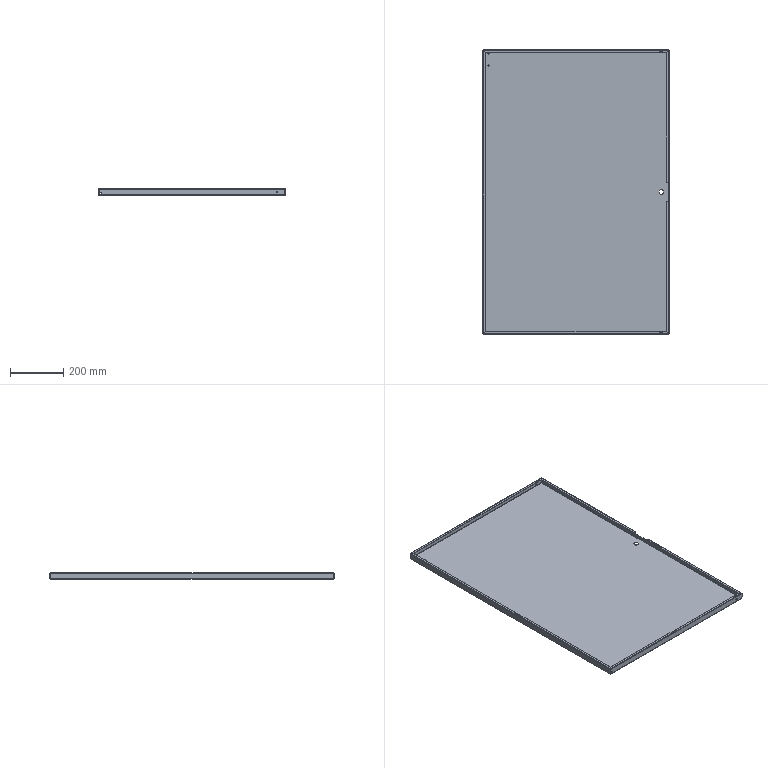Part | SolidWorks | features Cut 4, EdgeFlange 2, ICE 2, Fillet 1, FlatPattern 1, LPattern 1, MirrorPattern 1, SMBaseFlange 1, SheetMetal 1 | 1 solid | 110 faces | box 700 x 1066 x 25 mm | volume 1278991 mm3 | plane 52 | cylinder 42 | spline 16 | commonest cylinder face diameters 1.473 x9 4.473 x9 2.5 x8 5 x4 5.2 x4 6.3 x4